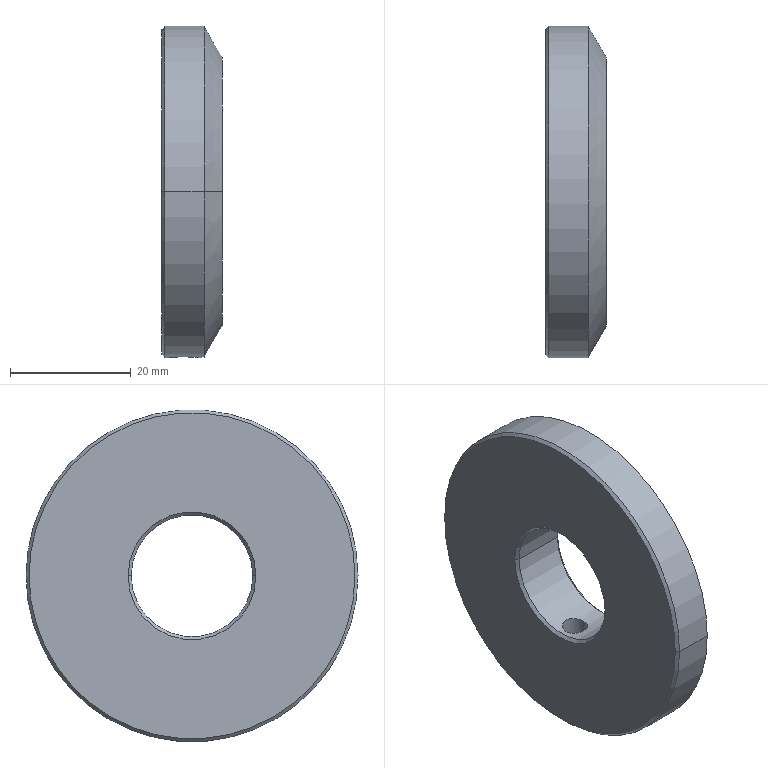Part | NX | 1 solid | 18 faces | box 10 x 55 x 55 mm | volume 19010 mm3 | cone 8 | cylinder 6 | plane 2 | spline 2 | commonest cylinder face diameters 4.2 x2 20.2 x2 55 x2
STEP:
#1=CARTESIAN_POINT('',(7.,27.5,0.));
#2=VERTEX_POINT('',#1);
#3=CARTESIAN_POINT('',(7.,-27.5,0.));
#4=VERTEX_POINT('',#3);
#5=CARTESIAN_POINT('',(7.,0.,0.));
#6=DIRECTION('',(-1.,0.,0.));
#7=DIRECTION('',(0.,1.,0.));
#8=AXIS2_PLACEMENT_3D('',#5,#6,#7);
#9=CIRCLE('',#8,27.5);
#10=EDGE_CURVE('',#2,#4,#9,.T.);
#11=ORIENTED_EDGE('',*,*,#10,.T.);
#12=CARTESIAN_POINT('',(0.5,-27.5,0.));
#13=VERTEX_POINT('',#12);
#14=CARTESIAN_POINT('',(0.,-27.5,0.));
#15=DIRECTION('',(1.,0.,0.));
#16=VECTOR('',#15,1000.);
#17=LINE('',#14,#16);
#18=EDGE_CURVE('',#4,#13,#17,.F.);
#19=ORIENTED_EDGE('',*,*,#18,.T.);
#20=CARTESIAN_POINT('',(0.5,27.5,0.));
#21=VERTEX_POINT('',#20);
#22=CARTESIAN_POINT('',(0.5,0.,0.));
#23=DIRECTION('',(1.,0.,0.));
#24=DIRECTION('',(0.,-1.,0.));
#25=AXIS2_PLACEMENT_3D('',#22,#23,#24);
#26=CIRCLE('',#25,27.5);
#27=EDGE_CURVE('',#13,#21,#26,.T.);
#28=ORIENTED_EDGE('',*,*,#27,.T.);
#29=CARTESIAN_POINT('',(0.,27.5,0.));
#30=DIRECTION('',(1.,0.,0.));
#31=VECTOR('',#30,1000.);
#32=LINE('',#29,#31);
#33=EDGE_CURVE('',#2,#21,#32,.F.);
#34=ORIENTED_EDGE('',*,*,#33,.F.);
#35=EDGE_LOOP('',(#11,#19,#28,#34));
#36=FACE_BOUND('',#35,.T.);
#37=CARTESIAN_POINT('',(6.36,-0.00005495,-27.5));
#38=VERTEX_POINT('',#37);
#39=CARTESIAN_POINT('',(0.64,-0.00002858,-27.5));
#40=VERTEX_POINT('',#39);
#41=CARTESIAN_POINT('',(6.36,-0.00005495,-27.5));
#42=CARTESIAN_POINT('',(6.36,0.7516,-27.5));
#43=CARTESIAN_POINT('',(5.681,2.206,-27.427));
#44=CARTESIAN_POINT('',(3.502,3.035,-27.329));
#45=CARTESIAN_POINT('',(1.317,2.208,-27.427));
#46=CARTESIAN_POINT('',(0.64,0.7456,-27.5));
#47=CARTESIAN_POINT('',(0.64,-0.00002858,-27.5));
#48=B_SPLINE_CURVE_WITH_KNOTS('',3,(#41,#42,#43,#44,#45,#46,#47),.UNSPECIFIED.,.F.,.F.,(4,1,1,1,4),(0.,0.25,0.5,0.75,1.),.UNSPECIFIED.);
#49=EDGE_CURVE('',#38,#40,#48,.T.);
#50=ORIENTED_EDGE('',*,*,#49,.T.);
#51=CARTESIAN_POINT('',(0.64,-0.00002858,-27.5));
#52=CARTESIAN_POINT('',(0.64,-0.7479,-27.5));
#53=CARTESIAN_POINT('',(1.32,-2.209,-27.426));
#54=CARTESIAN_POINT('',(3.501,-3.035,-27.329));
#55=CARTESIAN_POINT('',(5.684,-2.206,-27.427));
#56=CARTESIAN_POINT('',(6.359,-0.7474,-27.5));
#57=CARTESIAN_POINT('',(6.36,-0.00005495,-27.5));
#58=B_SPLINE_CURVE_WITH_KNOTS('',3,(#51,#52,#53,#54,#55,#56,#57),.UNSPECIFIED.,.F.,.F.,(4,1,1,1,4),(0.,0.25,0.5,0.75,1.),.UNSPECIFIED.);
#59=EDGE_CURVE('',#40,#38,#58,.T.);
#60=ORIENTED_EDGE('',*,*,#59,.T.);
#61=EDGE_LOOP('',(#50,#60));
#62=FACE_BOUND('',#61,.T.);
#63=CARTESIAN_POINT('',(0.,0.,0.));
#64=DIRECTION('',(1.,0.,0.));
#65=DIRECTION('',(0.,-1.,0.));
#66=AXIS2_PLACEMENT_3D('',#63,#64,#65);
#67=CYLINDRICAL_SURFACE('',#66,27.5);
#68=ADVANCED_FACE('',(#36,#62),#67,.T.);
#69=CARTESIAN_POINT('',(5.6,0.,-10.1));
#70=VERTEX_POINT('',#69);
#71=CARTESIAN_POINT('',(1.4,0.,-10.1));
#72=VERTEX_POINT('',#71);
#73=CARTESIAN_POINT('',(1.4,0.,-10.1));
#74=CARTESIAN_POINT('',(1.4,-0.2606,-10.1));
#75=CARTESIAN_POINT('',(1.513,-0.7432,-10.077));
#76=CARTESIAN_POINT('',(1.692,-1.088,-10.042));
#77=CARTESIAN_POINT('',(1.995,-1.502,-9.99));
#78=CARTESIAN_POINT('',(2.421,-1.814,-9.937));
#79=CARTESIAN_POINT('',(2.66,-1.936,-9.913));
#80=CARTESIAN_POINT('',(3.113,-2.082,-9.884));
#81=CARTESIAN_POINT('',(3.5,-2.109,-9.877));
#82=CARTESIAN_POINT('',(3.887,-2.082,-9.884));
#83=CARTESIAN_POINT('',(4.339,-1.936,-9.913));
#84=CARTESIAN_POINT('',(4.579,-1.814,-9.937));
#85=CARTESIAN_POINT('',(5.006,-1.502,-9.991));
#86=CARTESIAN_POINT('',(5.308,-1.089,-10.042));
#87=CARTESIAN_POINT('',(5.487,-0.7425,-10.077));
#88=CARTESIAN_POINT('',(5.6,-0.2606,-10.1));
#89=CARTESIAN_POINT('',(5.6,0.,-10.1));
#90=B_SPLINE_CURVE_WITH_KNOTS('',3,(#73,#74,#75,#76,#77,#78,#79,#80,#81,#82,#83,#84,#85,#86,#87,#88,#89),.UNSPECIFIED.,.F.,.F.,(4,1,1,1,1,1,1,1,1,1,1,1,1,1,4),(0.,0.125,0.1875,0.25,0.3125,0.375,0.4375,0.5,0.5625,0.625,0.6875,0.75,0.8125,0.875,1.),.UNSPECIFIED.);
#91=EDGE_CURVE('',#70,#72,#90,.F.);
#92=ORIENTED_EDGE('',*,*,#91,.F.);
#93=CARTESIAN_POINT('',(5.6,0.,-27.061));
#94=VERTEX_POINT('',#93);
#95=CARTESIAN_POINT('',(5.6,0.,-26.5));
#96=DIRECTION('',(0.,0.,-1.));
#97=VECTOR('',#96,1000.);
#98=LINE('',#95,#97);
#99=EDGE_CURVE('',#94,#70,#98,.F.);
#100=ORIENTED_EDGE('',*,*,#99,.F.);
#101=CARTESIAN_POINT('',(5.6,-0.001142,-27.061));
#102=VERTEX_POINT('',#101);
#103=CARTESIAN_POINT('',(5.6,0.,-27.061));
#104=CARTESIAN_POINT('',(5.6,-0.0003806,-27.061));
#105=CARTESIAN_POINT('',(5.6,-0.0007611,-27.061));
#106=CARTESIAN_POINT('',(5.6,-0.001142,-27.061));
#107=B_SPLINE_CURVE_WITH_KNOTS('',3,(#103,#104,#105,#106),.UNSPECIFIED.,.F.,.F.,(4,4),(0.,1.),.UNSPECIFIED.);
#108=EDGE_CURVE('',#102,#94,#107,.F.);
#109=ORIENTED_EDGE('',*,*,#108,.F.);
#110=CARTESIAN_POINT('',(1.4,0.,-27.061));
#111=VERTEX_POINT('',#110);
#112=CARTESIAN_POINT('',(5.6,-0.001142,-27.061));
#113=CARTESIAN_POINT('',(5.6,-0.2603,-27.061));
#114=CARTESIAN_POINT('',(5.489,-0.734,-27.053));
#115=CARTESIAN_POINT('',(5.318,-1.073,-27.04));
#116=CARTESIAN_POINT('',(5.016,-1.491,-27.021));
#117=CARTESIAN_POINT('',(4.596,-1.805,-27.002));
#118=CARTESIAN_POINT('',(4.348,-1.933,-26.993));
#119=CARTESIAN_POINT('',(3.897,-2.08,-26.983));
#120=CARTESIAN_POINT('',(3.501,-2.11,-26.98));
#121=CARTESIAN_POINT('',(3.103,-2.08,-26.983));
#122=CARTESIAN_POINT('',(2.653,-1.933,-26.993));
#123=CARTESIAN_POINT('',(2.405,-1.805,-27.002));
#124=CARTESIAN_POINT('',(1.985,-1.492,-27.021));
#125=CARTESIAN_POINT('',(1.684,-1.075,-27.04));
#126=CARTESIAN_POINT('',(1.512,-0.7359,-27.053));
#127=CARTESIAN_POINT('',(1.4,-0.2576,-27.061));
#128=CARTESIAN_POINT('',(1.4,0.,-27.061));
#129=B_SPLINE_CURVE_WITH_KNOTS('',3,(#112,#113,#114,#115,#116,#117,#118,#119,#120,#121,#122,#123,#124,#125,#126,#127,#128),.UNSPECIFIED.,.F.,.F.,(4,1,1,1,1,1,1,1,1,1,1,1,1,1,4),(0.,0.125,0.1875,0.25,0.3125,0.375,0.4375,0.5,0.5625,0.625,0.6875,0.75,0.8125,0.875,1.),.UNSPECIFIED.);
#130=EDGE_CURVE('',#111,#102,#129,.F.);
#131=ORIENTED_EDGE('',*,*,#130,.F.);
#132=CARTESIAN_POINT('',(1.4,0.,-26.5));
#133=DIRECTION('',(0.,0.,-1.));
#134=VECTOR('',#133,1000.);
#135=LINE('',#132,#134);
#136=EDGE_CURVE('',#111,#72,#135,.F.);
#137=ORIENTED_EDGE('',*,*,#136,.T.);
#138=EDGE_LOOP('',(#92,#100,#109,#131,#137));
#139=FACE_BOUND('',#138,.T.);
#140=CARTESIAN_POINT('',(3.5,0.,-26.5));
#141=DIRECTION('',(0.,0.,-1.));
#142=DIRECTION('',(-1.,0.,0.));
#143=AXIS2_PLACEMENT_3D('',#140,#141,#142);
#144=CYLINDRICAL_SURFACE('',#143,2.1);
#145=ADVANCED_FACE('',(#139),#144,.F.);
#146=ORIENTED_EDGE('',*,*,#10,.F.);
#147=CARTESIAN_POINT('',(10.,22.304,0.));
#148=VERTEX_POINT('',#147);
#149=CARTESIAN_POINT('',(8.5,24.902,0.));
#150=DIRECTION('',(-0.5,0.866,0.));
#151=VECTOR('',#150,1000.);
#152=LINE('',#149,#151);
#153=EDGE_CURVE('',#148,#2,#152,.T.);
#154=ORIENTED_EDGE('',*,*,#153,.F.);
#155=CARTESIAN_POINT('',(10.,-22.304,0.));
#156=VERTEX_POINT('',#155);
#157=CARTESIAN_POINT('',(10.,0.,0.));
#158=DIRECTION('',(-1.,0.,0.));
#159=DIRECTION('',(0.,1.,0.));
#160=AXIS2_PLACEMENT_3D('',#157,#158,#159);
#161=CIRCLE('',#160,22.304);
#162=EDGE_CURVE('',#148,#156,#161,.T.);
#163=ORIENTED_EDGE('',*,*,#162,.T.);
#164=CARTESIAN_POINT('',(8.5,-24.902,0.));
#165=DIRECTION('',(-0.5,-0.866,0.));
#166=VECTOR('',#165,1000.);
#167=LINE('',#164,#166);
#168=EDGE_CURVE('',#156,#4,#167,.T.);
#169=ORIENTED_EDGE('',*,*,#168,.T.);
#170=EDGE_LOOP('',(#146,#154,#163,#169));
#171=FACE_BOUND('',#170,.T.);
#172=CARTESIAN_POINT('',(8.5,0.,0.));
#173=DIRECTION('',(-1.,0.,0.));
#174=DIRECTION('',(0.,1.,0.));
#175=AXIS2_PLACEMENT_3D('',#172,#173,#174);
#176=CONICAL_SURFACE('',#175,24.902,1.047);
#177=ADVANCED_FACE('',(#171),#176,.T.);
#178=CARTESIAN_POINT('',(0.,27.,0.));
#179=VERTEX_POINT('',#178);
#180=CARTESIAN_POINT('',(0.,-27.,0.));
#181=VERTEX_POINT('',#180);
#182=CARTESIAN_POINT('',(0.,0.,0.));
#183=DIRECTION('',(1.,0.,0.));
#184=DIRECTION('',(0.,-1.,0.));
#185=AXIS2_PLACEMENT_3D('',#182,#183,#184);
#186=CIRCLE('',#185,27.);
#187=EDGE_CURVE('',#179,#181,#186,.T.);
#188=ORIENTED_EDGE('',*,*,#187,.F.);
#189=CARTESIAN_POINT('',(0.,0.,0.));
#190=DIRECTION('',(1.,0.,0.));
#191=DIRECTION('',(0.,-1.,0.));
#192=AXIS2_PLACEMENT_3D('',#189,#190,#191);
#193=CIRCLE('',#192,27.);
#194=EDGE_CURVE('',#181,#179,#193,.T.);
#195=ORIENTED_EDGE('',*,*,#194,.F.);
#196=EDGE_LOOP('',(#188,#195));
#197=FACE_BOUND('',#196,.T.);
#198=CARTESIAN_POINT('',(0.,-10.6,0.));
#199=VERTEX_POINT('',#198);
#200=CARTESIAN_POINT('',(0.,10.6,0.));
#201=VERTEX_POINT('',#200);
#202=CARTESIAN_POINT('',(0.,0.,0.));
#203=DIRECTION('',(-1.,0.,0.));
#204=DIRECTION('',(0.,1.,0.));
#205=AXIS2_PLACEMENT_3D('',#202,#203,#204);
#206=CIRCLE('',#205,10.6);
#207=EDGE_CURVE('',#199,#201,#206,.T.);
#208=ORIENTED_EDGE('',*,*,#207,.F.);
#209=CARTESIAN_POINT('',(0.,0.,0.));
#210=DIRECTION('',(-1.,0.,0.));
#211=DIRECTION('',(0.,1.,0.));
#212=AXIS2_PLACEMENT_3D('',#209,#210,#211);
#213=CIRCLE('',#212,10.6);
#214=EDGE_CURVE('',#201,#199,#213,.T.);
#215=ORIENTED_EDGE('',*,*,#214,.F.);
#216=EDGE_LOOP('',(#208,#215));
#217=FACE_BOUND('',#216,.T.);
#218=CARTESIAN_POINT('',(0.,0.,0.));
#219=DIRECTION('',(1.,0.,0.));
#220=DIRECTION('',(0.,1.,0.));
#221=AXIS2_PLACEMENT_3D('',#218,#219,#220);
#222=PLANE('',#221);
#223=ADVANCED_FACE('',(#197,#217),#222,.F.);
#224=CARTESIAN_POINT('',(10.,0.,0.));
#225=DIRECTION('',(-1.,0.,0.));
#226=DIRECTION('',(0.,1.,0.));
#227=AXIS2_PLACEMENT_3D('',#224,#225,#226);
#228=CIRCLE('',#227,22.304);
#229=EDGE_CURVE('',#156,#148,#228,.T.);
#230=ORIENTED_EDGE('',*,*,#229,.F.);
#231=ORIENTED_EDGE('',*,*,#162,.F.);
#232=EDGE_LOOP('',(#230,#231));
#233=FACE_BOUND('',#232,.T.);
#234=CARTESIAN_POINT('',(10.,10.6,0.));
#235=VERTEX_POINT('',#234);
#236=CARTESIAN_POINT('',(10.,-10.6,0.));
#237=VERTEX_POINT('',#236);
#238=CARTESIAN_POINT('',(10.,0.,0.));
#239=DIRECTION('',(1.,0.,0.));
#240=DIRECTION('',(0.,-1.,0.));
#241=AXIS2_PLACEMENT_3D('',#238,#239,#240);
#242=CIRCLE('',#241,10.6);
#243=EDGE_CURVE('',#235,#237,#242,.T.);
#244=ORIENTED_EDGE('',*,*,#243,.F.);
#245=CARTESIAN_POINT('',(10.,0.,0.));
#246=DIRECTION('',(1.,0.,0.));
#247=DIRECTION('',(0.,-1.,0.));
#248=AXIS2_PLACEMENT_3D('',#245,#246,#247);
#249=CIRCLE('',#248,10.6);
#250=EDGE_CURVE('',#237,#235,#249,.T.);
#251=ORIENTED_EDGE('',*,*,#250,.F.);
#252=EDGE_LOOP('',(#244,#251));
#253=FACE_BOUND('',#252,.T.);
#254=CARTESIAN_POINT('',(10.,0.,0.));
#255=DIRECTION('',(1.,0.,0.));
#256=DIRECTION('',(0.,1.,0.));
#257=AXIS2_PLACEMENT_3D('',#254,#255,#256);
#258=PLANE('',#257);
#259=ADVANCED_FACE('',(#233,#253),#258,.T.);
#260=CARTESIAN_POINT('',(0.5,10.1,0.));
#261=VERTEX_POINT('',#260);
#262=CARTESIAN_POINT('',(0.5,-10.1,0.));
#263=VERTEX_POINT('',#262);
#264=CARTESIAN_POINT('',(0.5,0.,0.));
#265=DIRECTION('',(-1.,0.,0.));
#266=DIRECTION('',(0.,1.,0.));
#267=AXIS2_PLACEMENT_3D('',#264,#265,#266);
#268=CIRCLE('',#267,10.1);
#269=EDGE_CURVE('',#261,#263,#268,.T.);
#270=ORIENTED_EDGE('',*,*,#269,.T.);
#271=CARTESIAN_POINT('',(9.5,-10.1,0.));
#272=VERTEX_POINT('',#271);
#273=CARTESIAN_POINT('',(0.,-10.1,0.));
#274=DIRECTION('',(1.,0.,0.));
#275=VECTOR('',#274,1000.);
#276=LINE('',#273,#275);
#277=EDGE_CURVE('',#272,#263,#276,.F.);
#278=ORIENTED_EDGE('',*,*,#277,.F.);
#279=CARTESIAN_POINT('',(9.5,10.1,0.));
#280=VERTEX_POINT('',#279);
#281=CARTESIAN_POINT('',(9.5,0.,0.));
#282=DIRECTION('',(1.,0.,0.));
#283=DIRECTION('',(0.,-1.,0.));
#284=AXIS2_PLACEMENT_3D('',#281,#282,#283);
#285=CIRCLE('',#284,10.1);
#286=EDGE_CURVE('',#272,#280,#285,.T.);
#287=ORIENTED_EDGE('',*,*,#286,.T.);
#288=CARTESIAN_POINT('',(0.,10.1,0.));
#289=DIRECTION('',(1.,0.,0.));
#290=VECTOR('',#289,1000.);
#291=LINE('',#288,#290);
#292=EDGE_CURVE('',#280,#261,#291,.F.);
#293=ORIENTED_EDGE('',*,*,#292,.T.);
#294=EDGE_LOOP('',(#270,#278,#287,#293));
#295=FACE_BOUND('',#294,.T.);
#296=CARTESIAN_POINT('',(3.5,2.1,-9.879));
#297=VERTEX_POINT('',#296);
#298=CARTESIAN_POINT('',(1.4,0.,-10.1));
#299=CARTESIAN_POINT('',(1.4,1.115,-10.1));
#300=CARTESIAN_POINT('',(2.384,2.099,-9.879));
#301=CARTESIAN_POINT('',(3.5,2.1,-9.879));
#302=B_SPLINE_CURVE_WITH_KNOTS('',3,(#298,#299,#300,#301),.UNSPECIFIED.,.F.,.F.,(4,4),(0.,1.),.UNSPECIFIED.);
#303=EDGE_CURVE('',#72,#297,#302,.T.);
#304=ORIENTED_EDGE('',*,*,#303,.T.);
#305=CARTESIAN_POINT('',(3.5,2.1,-9.879));
#306=CARTESIAN_POINT('',(4.615,2.099,-9.879));
#307=CARTESIAN_POINT('',(5.6,1.115,-10.1));
#308=CARTESIAN_POINT('',(5.6,0.,-10.1));
#309=B_SPLINE_CURVE_WITH_KNOTS('',3,(#305,#306,#307,#308),.UNSPECIFIED.,.F.,.F.,(4,4),(0.,1.),.UNSPECIFIED.);
#310=EDGE_CURVE('',#297,#70,#309,.T.);
#311=ORIENTED_EDGE('',*,*,#310,.T.);
#312=ORIENTED_EDGE('',*,*,#91,.T.);
#313=EDGE_LOOP('',(#304,#311,#312));
#314=FACE_BOUND('',#313,.T.);
#315=CARTESIAN_POINT('',(0.,0.,0.));
#316=DIRECTION('',(1.,0.,0.));
#317=DIRECTION('',(0.,-1.,0.));
#318=AXIS2_PLACEMENT_3D('',#315,#316,#317);
#319=CYLINDRICAL_SURFACE('',#318,10.1);
#320=ADVANCED_FACE('',(#295,#314),#319,.F.);
#321=ORIENTED_EDGE('',*,*,#286,.F.);
#322=CARTESIAN_POINT('',(10.,-10.6,0.));
#323=DIRECTION('',(0.7071,-0.7071,0.));
#324=VECTOR('',#323,1000.);
#325=LINE('',#322,#324);
#326=EDGE_CURVE('',#237,#272,#325,.F.);
#327=ORIENTED_EDGE('',*,*,#326,.F.);
#328=ORIENTED_EDGE('',*,*,#250,.T.);
#329=CARTESIAN_POINT('',(10.,10.6,0.));
#330=DIRECTION('',(0.7071,0.7071,0.));
#331=VECTOR('',#330,1000.);
#332=LINE('',#329,#331);
#333=EDGE_CURVE('',#235,#280,#332,.F.);
#334=ORIENTED_EDGE('',*,*,#333,.T.);
#335=EDGE_LOOP('',(#321,#327,#328,#334));
#336=FACE_BOUND('',#335,.T.);
#337=CARTESIAN_POINT('',(10.,0.,0.));
#338=DIRECTION('',(1.,0.,0.));
#339=DIRECTION('',(0.,-1.,0.));
#340=AXIS2_PLACEMENT_3D('',#337,#338,#339);
#341=CONICAL_SURFACE('',#340,10.6,0.7854);
#342=ADVANCED_FACE('',(#336),#341,.F.);
#343=ORIENTED_EDGE('',*,*,#207,.T.);
#344=CARTESIAN_POINT('',(0.,10.6,0.));
#345=DIRECTION('',(-0.7071,0.7071,0.));
#346=VECTOR('',#345,1000.);
#347=LINE('',#344,#346);
#348=EDGE_CURVE('',#261,#201,#347,.T.);
#349=ORIENTED_EDGE('',*,*,#348,.F.);
#350=CARTESIAN_POINT('',(0.5,0.,0.));
#351=DIRECTION('',(-1.,0.,0.));
#352=DIRECTION('',(0.,1.,0.));
#353=AXIS2_PLACEMENT_3D('',#350,#351,#352);
#354=CIRCLE('',#353,10.1);
#355=EDGE_CURVE('',#263,#261,#354,.T.);
#356=ORIENTED_EDGE('',*,*,#355,.F.);
#357=CARTESIAN_POINT('',(0.,-10.6,0.));
#358=DIRECTION('',(-0.7071,-0.7071,0.));
#359=VECTOR('',#358,1000.);
#360=LINE('',#357,#359);
#361=EDGE_CURVE('',#263,#199,#360,.T.);
#362=ORIENTED_EDGE('',*,*,#361,.T.);
#363=EDGE_LOOP('',(#343,#349,#356,#362));
#364=FACE_BOUND('',#363,.T.);
#365=CARTESIAN_POINT('',(0.,0.,0.));
#366=DIRECTION('',(-1.,0.,0.));
#367=DIRECTION('',(0.,1.,0.));
#368=AXIS2_PLACEMENT_3D('',#365,#366,#367);
#369=CONICAL_SURFACE('',#368,10.6,0.7854);
#370=ADVANCED_FACE('',(#364),#369,.F.);
#371=ORIENTED_EDGE('',*,*,#130,.T.);
#372=ORIENTED_EDGE('',*,*,#108,.T.);
#373=CARTESIAN_POINT('',(5.6,0.000000116,-27.061));
#374=CARTESIAN_POINT('',(5.853,0.00004363,-27.207));
#375=CARTESIAN_POINT('',(6.106,0.00002528,-27.354));
#376=CARTESIAN_POINT('',(6.36,-0.00005495,-27.5));
#377=B_SPLINE_CURVE_WITH_KNOTS('',3,(#373,#374,#375,#376),.UNSPECIFIED.,.F.,.F.,(4,4),(0.,1.),.UNSPECIFIED.);
#378=EDGE_CURVE('',#94,#38,#377,.T.);
#379=ORIENTED_EDGE('',*,*,#378,.T.);
#380=ORIENTED_EDGE('',*,*,#59,.F.);
#381=CARTESIAN_POINT('',(1.4,0.,-27.061));
#382=CARTESIAN_POINT('',(0.64,-0.00002858,-27.5));
#383=B_SPLINE_CURVE_WITH_KNOTS('',1,(#381,#382),.UNSPECIFIED.,.F.,.F.,(2,2),(0.,1.),.UNSPECIFIED.);
#384=EDGE_CURVE('',#111,#40,#383,.T.);
#385=ORIENTED_EDGE('',*,*,#384,.F.);
#386=EDGE_LOOP('',(#371,#372,#379,#380,#385));
#387=FACE_BOUND('',#386,.T.);
#388=CARTESIAN_POINT('',(1.4,0.03926,-27.061));
#389=CARTESIAN_POINT('',(0.64,0.05394,-27.5));
#390=CARTESIAN_POINT('',(1.4,0.02616,-27.061));
#391=CARTESIAN_POINT('',(0.64,0.03595,-27.5));
#392=CARTESIAN_POINT('',(1.4,0.01307,-27.061));
#393=CARTESIAN_POINT('',(0.64,0.01796,-27.5));
#394=CARTESIAN_POINT('',(1.4,-0.00002079,-27.061));
#395=CARTESIAN_POINT('',(0.64,-0.00002858,-27.5));
#396=CARTESIAN_POINT('',(1.4,-0.2204,-27.061));
#397=CARTESIAN_POINT('',(0.64,-0.3029,-27.5));
#398=CARTESIAN_POINT('',(1.434,-0.4384,-27.058));
#399=CARTESIAN_POINT('',(0.6927,-0.605,-27.495));
#400=CARTESIAN_POINT('',(1.61,-0.9776,-27.046));
#401=CARTESIAN_POINT('',(0.9515,-1.334,-27.471));
#402=CARTESIAN_POINT('',(1.796,-1.276,-27.032));
#403=CARTESIAN_POINT('',(1.223,-1.728,-27.447));
#404=CARTESIAN_POINT('',(2.301,-1.759,-27.006));
#405=CARTESIAN_POINT('',(1.924,-2.345,-27.402));
#406=CARTESIAN_POINT('',(2.614,-1.936,-26.993));
#407=CARTESIAN_POINT('',(2.341,-2.56,-27.381));
#408=CARTESIAN_POINT('',(3.298,-2.12,-26.98));
#409=CARTESIAN_POINT('',(3.24,-2.784,-27.359));
#410=CARTESIAN_POINT('',(3.661,-2.124,-26.979));
#411=CARTESIAN_POINT('',(3.706,-2.788,-27.359));
#412=CARTESIAN_POINT('',(4.348,-1.953,-26.992));
#413=CARTESIAN_POINT('',(4.609,-2.581,-27.379));
#414=CARTESIAN_POINT('',(4.664,-1.782,-27.004));
#415=CARTESIAN_POINT('',(5.029,-2.373,-27.399));
#416=CARTESIAN_POINT('',(5.178,-1.309,-27.031));
#417=CARTESIAN_POINT('',(5.74,-1.771,-27.445));
#418=CARTESIAN_POINT('',(5.37,-1.015,-27.044));
#419=CARTESIAN_POINT('',(6.019,-1.385,-27.469));
#420=CARTESIAN_POINT('',(5.561,-0.4662,-27.058));
#421=CARTESIAN_POINT('',(6.301,-0.6432,-27.494));
#422=CARTESIAN_POINT('',(5.6,-0.234,-27.061));
#423=CARTESIAN_POINT('',(6.359,-0.322,-27.5));
#424=CARTESIAN_POINT('',(5.6,-0.0004898,-27.061));
#425=CARTESIAN_POINT('',(6.36,-0.00005495,-27.5));
#426=CARTESIAN_POINT('',(5.6,0.01265,-27.061));
#427=CARTESIAN_POINT('',(6.36,0.01806,-27.5));
#428=CARTESIAN_POINT('',(5.6,0.02578,-27.061));
#429=CARTESIAN_POINT('',(6.36,0.03617,-27.5));
#430=CARTESIAN_POINT('',(5.6,0.03892,-27.061));
#431=CARTESIAN_POINT('',(6.36,0.05429,-27.5));
#432=B_SPLINE_SURFACE_WITH_KNOTS('',3,1,((#388,#389),(#390,#391),(#392,#393),(#394,#395),(#396,#397),(#398,#399),(#400,#401),(#402,#403),(#404,#405),(#406,#407),(#408,#409),(#410,#411),(#412,#413),(#414,#415),(#416,#417),(#418,#419),(#420,#421),(#422,#423),(#424,#425),(#426,#427),(#428,#429),(#430,#431)),.RULED_SURF.,.F.,.F.,.F.,(4,3,2,2,2,2,2,2,3,4),(2,2),(-0.04652,0.,0.7833,2.008,3.235,4.464,5.69,6.912,7.749,7.796),(0.,1.),.UNSPECIFIED.);
#433=ADVANCED_FACE('',(#387),#432,.T.);
#434=ORIENTED_EDGE('',*,*,#187,.T.);
#435=CARTESIAN_POINT('',(0.,-27.,0.));
#436=DIRECTION('',(0.7071,-0.7071,0.));
#437=VECTOR('',#436,1000.);
#438=LINE('',#435,#437);
#439=EDGE_CURVE('',#13,#181,#438,.F.);
#440=ORIENTED_EDGE('',*,*,#439,.F.);
#441=CARTESIAN_POINT('',(0.5,0.,0.));
#442=DIRECTION('',(1.,0.,0.));
#443=DIRECTION('',(0.,-1.,0.));
#444=AXIS2_PLACEMENT_3D('',#441,#442,#443);
#445=CIRCLE('',#444,27.5);
#446=EDGE_CURVE('',#21,#13,#445,.T.);
#447=ORIENTED_EDGE('',*,*,#446,.F.);
#448=CARTESIAN_POINT('',(0.,27.,0.));
#449=DIRECTION('',(0.7071,0.7071,0.));
#450=VECTOR('',#449,1000.);
#451=LINE('',#448,#450);
#452=EDGE_CURVE('',#21,#179,#451,.F.);
#453=ORIENTED_EDGE('',*,*,#452,.T.);
#454=EDGE_LOOP('',(#434,#440,#447,#453));
#455=FACE_BOUND('',#454,.T.);
#456=CARTESIAN_POINT('',(0.,0.,0.));
#457=DIRECTION('',(1.,0.,0.));
#458=DIRECTION('',(0.,-1.,0.));
#459=AXIS2_PLACEMENT_3D('',#456,#457,#458);
#460=CONICAL_SURFACE('',#459,27.,0.7854);
#461=ADVANCED_FACE('',(#455),#460,.T.);
#462=ORIENTED_EDGE('',*,*,#136,.F.);
#463=CARTESIAN_POINT('',(1.4,0.,-27.061));
#464=CARTESIAN_POINT('',(1.4,0.2536,-27.061));
#465=CARTESIAN_POINT('',(1.511,0.7345,-27.053));
#466=CARTESIAN_POINT('',(1.681,1.07,-27.04));
#467=CARTESIAN_POINT('',(1.984,1.492,-27.021));
#468=CARTESIAN_POINT('',(2.407,1.806,-27.002));
#469=CARTESIAN_POINT('',(2.65,1.932,-26.993));
#470=CARTESIAN_POINT('',(3.112,2.082,-26.982));
#471=CARTESIAN_POINT('',(3.498,2.109,-26.98));
#472=CARTESIAN_POINT('',(3.896,2.081,-26.983));
#473=CARTESIAN_POINT('',(4.349,1.932,-26.993));
#474=CARTESIAN_POINT('',(4.588,1.809,-27.002));
#475=CARTESIAN_POINT('',(5.017,1.491,-27.021));
#476=CARTESIAN_POINT('',(5.316,1.076,-27.04));
#477=CARTESIAN_POINT('',(5.49,0.7332,-27.053));
#478=CARTESIAN_POINT('',(5.6,0.2552,-27.061));
#479=CARTESIAN_POINT('',(5.6,0.,-27.061));
#480=B_SPLINE_CURVE_WITH_KNOTS('',3,(#463,#464,#465,#466,#467,#468,#469,#470,#471,#472,#473,#474,#475,#476,#477,#478,#479),.UNSPECIFIED.,.F.,.F.,(4,1,1,1,1,1,1,1,1,1,1,1,1,1,4),(0.,0.125,0.1875,0.25,0.3125,0.375,0.4375,0.5,0.5625,0.625,0.6875,0.75,0.8125,0.875,1.),.UNSPECIFIED.);
#481=EDGE_CURVE('',#94,#111,#480,.F.);
#482=ORIENTED_EDGE('',*,*,#481,.F.);
#483=ORIENTED_EDGE('',*,*,#99,.T.);
#484=ORIENTED_EDGE('',*,*,#310,.F.);
#485=ORIENTED_EDGE('',*,*,#303,.F.);
#486=EDGE_LOOP('',(#462,#482,#483,#484,#485));
#487=FACE_BOUND('',#486,.T.);
#488=CARTESIAN_POINT('',(3.5,0.,-26.5));
#489=DIRECTION('',(0.,0.,-1.));
#490=DIRECTION('',(-1.,0.,0.));
#491=AXIS2_PLACEMENT_3D('',#488,#489,#490);
#492=CYLINDRICAL_SURFACE('',#491,2.1);
#493=ADVANCED_FACE('',(#487),#492,.F.);
#494=ORIENTED_EDGE('',*,*,#269,.F.);
#495=ORIENTED_EDGE('',*,*,#348,.T.);
#496=ORIENTED_EDGE('',*,*,#214,.T.);
#497=ORIENTED_EDGE('',*,*,#361,.F.);
#498=EDGE_LOOP('',(#494,#495,#496,#497));
#499=FACE_BOUND('',#498,.T.);
#500=CARTESIAN_POINT('',(0.,0.,0.));
#501=DIRECTION('',(-1.,0.,0.));
#502=DIRECTION('',(0.,1.,0.));
#503=AXIS2_PLACEMENT_3D('',#500,#501,#502);
#504=CONICAL_SURFACE('',#503,10.6,0.7854);
#505=ADVANCED_FACE('',(#499),#504,.F.);
#506=ORIENTED_EDGE('',*,*,#243,.T.);
#507=ORIENTED_EDGE('',*,*,#326,.T.);
#508=CARTESIAN_POINT('',(9.5,0.,0.));
#509=DIRECTION('',(1.,0.,0.));
#510=DIRECTION('',(0.,-1.,0.));
#511=AXIS2_PLACEMENT_3D('',#508,#509,#510);
#512=CIRCLE('',#511,10.1);
#513=EDGE_CURVE('',#280,#272,#512,.T.);
#514=ORIENTED_EDGE('',*,*,#513,.F.);
#515=ORIENTED_EDGE('',*,*,#333,.F.);
#516=EDGE_LOOP('',(#506,#507,#514,#515));
#517=FACE_BOUND('',#516,.T.);
#518=CARTESIAN_POINT('',(10.,0.,0.));
#519=DIRECTION('',(1.,0.,0.));
#520=DIRECTION('',(0.,-1.,0.));
#521=AXIS2_PLACEMENT_3D('',#518,#519,#520);
#522=CONICAL_SURFACE('',#521,10.6,0.7854);
#523=ADVANCED_FACE('',(#517),#522,.F.);
#524=ORIENTED_EDGE('',*,*,#18,.F.);
#525=CARTESIAN_POINT('',(7.,0.,0.));
#526=DIRECTION('',(-1.,0.,0.));
#527=DIRECTION('',(0.,1.,0.));
#528=AXIS2_PLACEMENT_3D('',#525,#526,#527);
#529=CIRCLE('',#528,27.5);
#530=EDGE_CURVE('',#4,#2,#529,.T.);
#531=ORIENTED_EDGE('',*,*,#530,.T.);
#532=ORIENTED_EDGE('',*,*,#33,.T.);
#533=ORIENTED_EDGE('',*,*,#446,.T.);
#534=EDGE_LOOP('',(#524,#531,#532,#533));
#535=FACE_BOUND('',#534,.T.);
#536=CARTESIAN_POINT('',(0.,0.,0.));
#537=DIRECTION('',(1.,0.,0.));
#538=DIRECTION('',(0.,-1.,0.));
#539=AXIS2_PLACEMENT_3D('',#536,#537,#538);
#540=CYLINDRICAL_SURFACE('',#539,27.5);
#541=ADVANCED_FACE('',(#535),#540,.T.);
#542=ORIENTED_EDGE('',*,*,#27,.F.);
#543=ORIENTED_EDGE('',*,*,#439,.T.);
#544=ORIENTED_EDGE('',*,*,#194,.T.);
#545=ORIENTED_EDGE('',*,*,#452,.F.);
#546=EDGE_LOOP('',(#542,#543,#544,#545));
#547=FACE_BOUND('',#546,.T.);
#548=CARTESIAN_POINT('',(0.,0.,0.));
#549=DIRECTION('',(1.,0.,0.));
#550=DIRECTION('',(0.,-1.,0.));
#551=AXIS2_PLACEMENT_3D('',#548,#549,#550);
#552=CONICAL_SURFACE('',#551,27.,0.7854);
#553=ADVANCED_FACE('',(#547),#552,.T.);
#554=ORIENTED_EDGE('',*,*,#277,.T.);
#555=ORIENTED_EDGE('',*,*,#355,.T.);
#556=ORIENTED_EDGE('',*,*,#292,.F.);
#557=ORIENTED_EDGE('',*,*,#513,.T.);
#558=EDGE_LOOP('',(#554,#555,#556,#557));
#559=FACE_BOUND('',#558,.T.);
#560=CARTESIAN_POINT('',(0.,0.,0.));
#561=DIRECTION('',(1.,0.,0.));
#562=DIRECTION('',(0.,-1.,0.));
#563=AXIS2_PLACEMENT_3D('',#560,#561,#562);
#564=CYLINDRICAL_SURFACE('',#563,10.1);
#565=ADVANCED_FACE('',(#559),#564,.F.);
#566=ORIENTED_EDGE('',*,*,#229,.T.);
#567=ORIENTED_EDGE('',*,*,#153,.T.);
#568=ORIENTED_EDGE('',*,*,#530,.F.);
#569=ORIENTED_EDGE('',*,*,#168,.F.);
#570=EDGE_LOOP('',(#566,#567,#568,#569));
#571=FACE_BOUND('',#570,.T.);
#572=CARTESIAN_POINT('',(8.5,0.,0.));
#573=DIRECTION('',(-1.,0.,0.));
#574=DIRECTION('',(0.,1.,0.));
#575=AXIS2_PLACEMENT_3D('',#572,#573,#574);
#576=CONICAL_SURFACE('',#575,24.902,1.047);
#577=ADVANCED_FACE('',(#571),#576,.T.);
#578=ORIENTED_EDGE('',*,*,#378,.F.);
#579=ORIENTED_EDGE('',*,*,#481,.T.);
#580=ORIENTED_EDGE('',*,*,#384,.T.);
#581=ORIENTED_EDGE('',*,*,#49,.F.);
#582=EDGE_LOOP('',(#578,#579,#580,#581));
#583=FACE_BOUND('',#582,.T.);
#584=CARTESIAN_POINT('',(5.6,-0.0004898,-27.061));
#585=CARTESIAN_POINT('',(6.36,-0.00005495,-27.5));
#586=CARTESIAN_POINT('',(5.6,0.1074,-27.061));
#587=CARTESIAN_POINT('',(6.36,0.1488,-27.5));
#588=CARTESIAN_POINT('',(5.592,0.2156,-27.061));
#589=CARTESIAN_POINT('',(6.347,0.2977,-27.499));
#590=CARTESIAN_POINT('',(5.522,0.6659,-27.055));
#591=CARTESIAN_POINT('',(6.242,0.9135,-27.489));
#592=CARTESIAN_POINT('',(5.385,0.9895,-27.045));
#593=CARTESIAN_POINT('',(6.037,1.352,-27.469));
#594=CARTESIAN_POINT('',(4.964,1.545,-27.019));
#595=CARTESIAN_POINT('',(5.44,2.075,-27.424));
#596=CARTESIAN_POINT('',(4.686,1.768,-27.004));
#597=CARTESIAN_POINT('',(5.06,2.353,-27.4));
#598=CARTESIAN_POINT('',(4.046,2.058,-26.984));
#599=CARTESIAN_POINT('',(4.207,2.71,-27.367));
#600=CARTESIAN_POINT('',(3.69,2.121,-26.979));
#601=CARTESIAN_POINT('',(3.749,2.784,-27.359));
#602=CARTESIAN_POINT('',(2.984,2.066,-26.983));
#603=CARTESIAN_POINT('',(2.827,2.718,-27.365));
#604=CARTESIAN_POINT('',(2.641,1.949,-26.993));
#605=CARTESIAN_POINT('',(2.38,2.578,-27.38));
#606=CARTESIAN_POINT('',(2.052,1.561,-27.017));
#607=CARTESIAN_POINT('',(1.583,2.094,-27.421));
#608=CARTESIAN_POINT('',(1.813,1.298,-27.032));
#609=CARTESIAN_POINT('',(1.246,1.757,-27.447));
#610=CARTESIAN_POINT('',(1.485,0.6847,-27.054));
#611=CARTESIAN_POINT('',(0.77,0.9429,-27.487));
#612=CARTESIAN_POINT('',(1.4,0.3458,-27.061));
#613=CARTESIAN_POINT('',(0.64,0.4751,-27.5));
#614=CARTESIAN_POINT('',(1.4,-0.00002079,-27.061));
#615=CARTESIAN_POINT('',(0.64,-0.00002858,-27.5));
#616=B_SPLINE_SURFACE_WITH_KNOTS('',3,1,((#584,#585),(#586,#587),(#588,#589),(#590,#591),(#592,#593),(#594,#595),(#596,#597),(#598,#599),(#600,#601),(#602,#603),(#604,#605),(#606,#607),(#608,#609),(#610,#611),(#612,#613),(#614,#615)),.RULED_SURF.,.F.,.F.,.F.,(4,2,2,2,2,2,2,4),(2,2),(7.749,8.136,9.366,10.589,11.811,13.041,14.27,15.498),(0.,1.),.UNSPECIFIED.);
#617=ADVANCED_FACE('',(#583),#616,.T.);
#618=CLOSED_SHELL('',(#68,#145,#177,#223,#259,#320,#342,#370,#433,#461,#493,#505,#523,#541,#553,#565,#577,#617));
#619=MANIFOLD_SOLID_BREP('',#618);
#620=(LENGTH_UNIT()NAMED_UNIT(*)SI_UNIT(.MILLI.,.METRE.));
#621=UNCERTAINTY_MEASURE_WITH_UNIT(LENGTH_MEASURE(0.0508),#620,'','');
#622=(NAMED_UNIT(*)PLANE_ANGLE_UNIT()SI_UNIT($,.RADIAN.));
#623=(NAMED_UNIT(*)SI_UNIT($,.STERADIAN.)SOLID_ANGLE_UNIT());
#624=(GEOMETRIC_REPRESENTATION_CONTEXT(3)GLOBAL_UNCERTAINTY_ASSIGNED_CONTEXT((#621))GLOBAL_UNIT_ASSIGNED_CONTEXT((#620,#622,#623))REPRESENTATION_CONTEXT('',''));
#625=ADVANCED_BREP_SHAPE_REPRESENTATION('',(#619),#624);